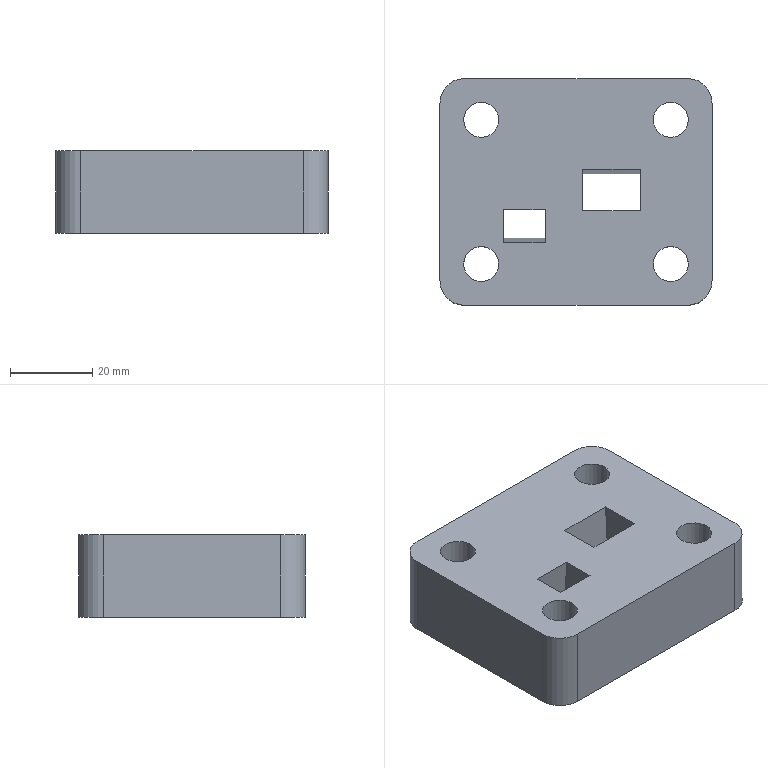Part | STEP file | solid 89 | 1 solid | 37 faces | box 66 x 55 x 20 mm | volume 59537 mm3 | plane 23 | cylinder 12 | other 2 | commonest cylinder face diameters 8.5 x4 12 x4 14 x4